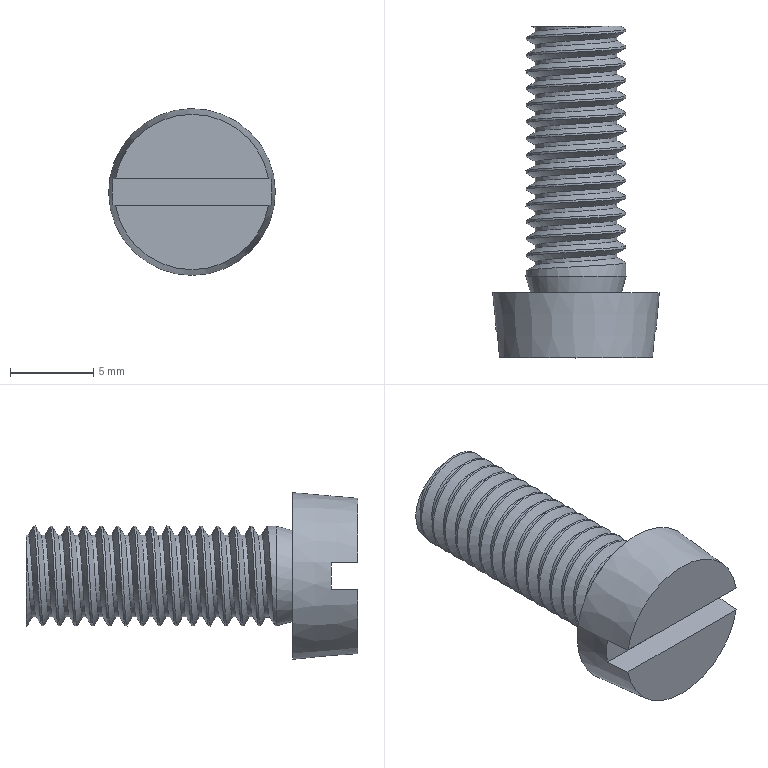Part | NX | features DATUM_CSYS 3, SKETCH 2, EXTRUDE 1, SWP104 1, THREADS 1 | 1 solid | 14 faces | box 10 x 19.9 x 10 mm | volume 653.386 mm3 | plane 8 | cone 2 | cylinder 2 | spline 2 | commonest cylinder face diameters 4.918 x1 6 x1